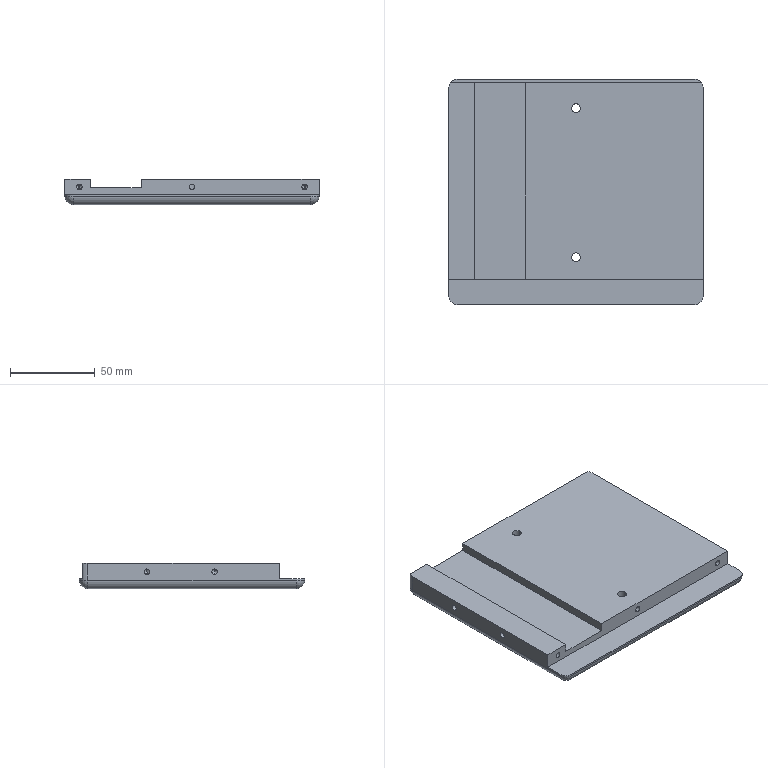Part | SolidWorks | features HoleWzd 4, ICE 3, Extrusion 1, Fillet 1, MirrorPattern 1 | 1 solid | 72 faces | box 150 x 133 x 15 mm | volume 253404 mm3 | cylinder 36 | cone 16 | plane 16 | sphere 4 | commonest cylinder face diameters 3.3 x20 10 x12 5.3 x4